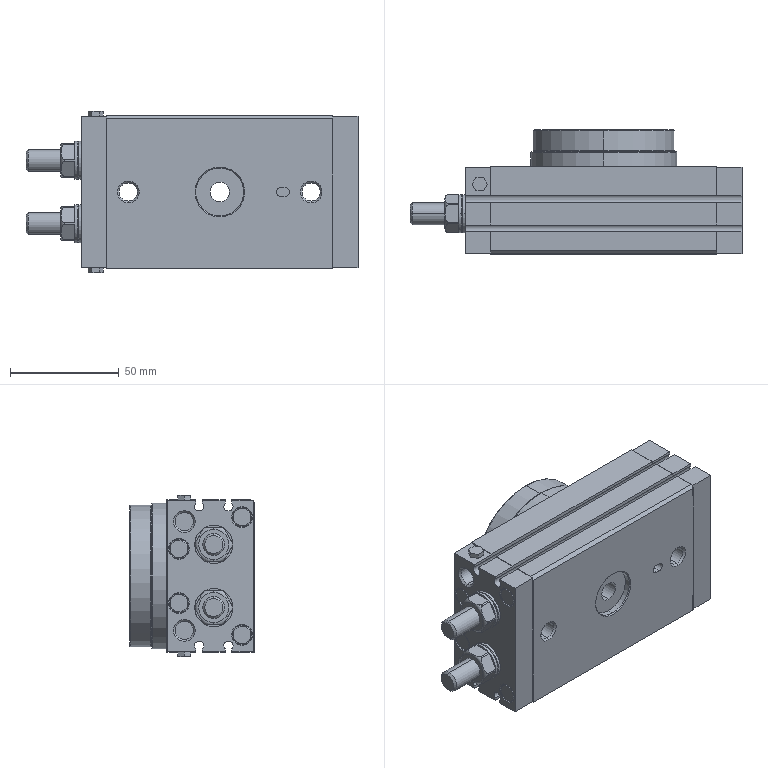Part | SolidWorks | 1 solid | 440 faces | box 152.5 x 57 x 74 mm | volume 389553 mm3 | plane 154 | cylinder 146 | cone 126 | torus 14 | commonest cylinder face diameters 4.917 x24 8.5 x20 9 x18 2.622 x12 7.78 x12 8.28 x12